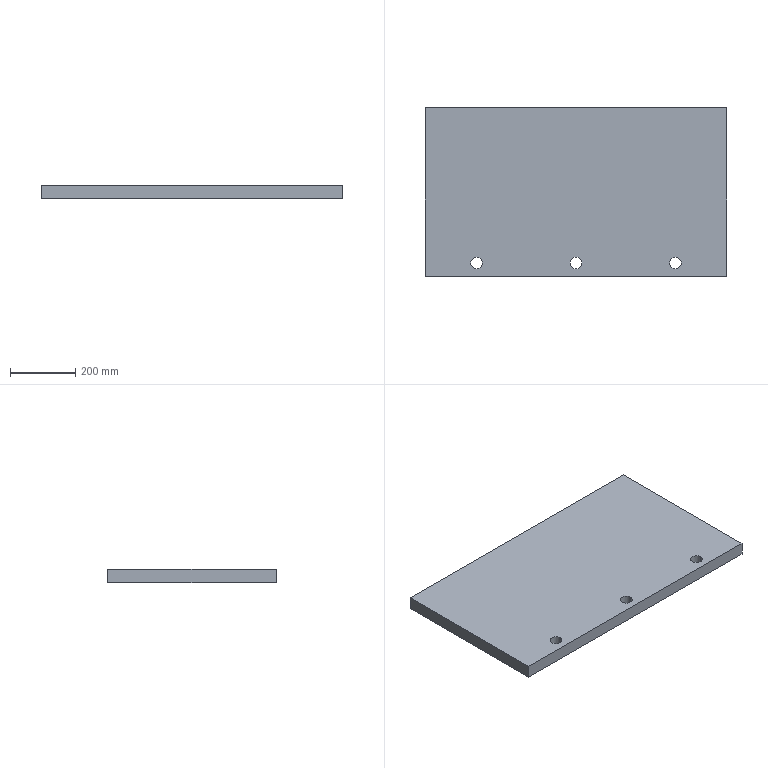Part | SolidWorks | features Extrusion 1 | 1 solid | 12 faces | box 922 x 515 x 40 mm | volume 18871055 mm3 | cylinder 6 | plane 6 | commonest cylinder face diameters 36 x6
STEP:
#1=CARTESIAN_POINT('',(139.,40.,40.));
#2=VERTEX_POINT('',#1);
#3=CARTESIAN_POINT('',(175.,40.,40.));
#4=VERTEX_POINT('',#3);
#5=CARTESIAN_POINT('',(157.,40.,40.));
#6=DIRECTION('',(0.,0.,1.));
#7=DIRECTION('',(1.,0.,0.));
#8=AXIS2_PLACEMENT_3D('',#5,#6,#7);
#9=CIRCLE('',#8,18.);
#10=EDGE_CURVE('',#2,#4,#9,.T.);
#11=ORIENTED_EDGE('',*,*,#10,.T.);
#12=CARTESIAN_POINT('',(175.,40.,0.));
#13=VERTEX_POINT('',#12);
#14=CARTESIAN_POINT('',(175.,40.,40.));
#15=DIRECTION('',(0.,0.,-1.));
#16=VECTOR('',#15,1000.);
#17=LINE('',#14,#16);
#18=EDGE_CURVE('',#4,#13,#17,.T.);
#19=ORIENTED_EDGE('',*,*,#18,.T.);
#20=CARTESIAN_POINT('',(139.,40.,0.));
#21=VERTEX_POINT('',#20);
#22=CARTESIAN_POINT('',(157.,40.,0.));
#23=DIRECTION('',(0.,0.,1.));
#24=DIRECTION('',(1.,0.,0.));
#25=AXIS2_PLACEMENT_3D('',#22,#23,#24);
#26=CIRCLE('',#25,18.);
#27=EDGE_CURVE('',#21,#13,#26,.T.);
#28=ORIENTED_EDGE('',*,*,#27,.F.);
#29=CARTESIAN_POINT('',(139.,40.,40.));
#30=DIRECTION('',(0.,0.,-1.));
#31=VECTOR('',#30,1000.);
#32=LINE('',#29,#31);
#33=EDGE_CURVE('',#2,#21,#32,.T.);
#34=ORIENTED_EDGE('',*,*,#33,.F.);
#35=EDGE_LOOP('',(#11,#19,#28,#34));
#36=FACE_OUTER_BOUND('',#35,.T.);
#37=CARTESIAN_POINT('',(157.,40.,40.));
#38=DIRECTION('',(0.,0.,-1.));
#39=DIRECTION('',(-1.,0.,0.));
#40=AXIS2_PLACEMENT_3D('',#37,#38,#39);
#41=CYLINDRICAL_SURFACE('',#40,18.);
#42=ADVANCED_FACE('',(#36),#41,.F.);
#43=CARTESIAN_POINT('',(747.,40.,40.));
#44=VERTEX_POINT('',#43);
#45=CARTESIAN_POINT('',(783.,40.,40.));
#46=VERTEX_POINT('',#45);
#47=CARTESIAN_POINT('',(765.,40.,40.));
#48=DIRECTION('',(0.,0.,1.));
#49=DIRECTION('',(1.,0.,0.));
#50=AXIS2_PLACEMENT_3D('',#47,#48,#49);
#51=CIRCLE('',#50,18.);
#52=EDGE_CURVE('',#44,#46,#51,.T.);
#53=ORIENTED_EDGE('',*,*,#52,.T.);
#54=CARTESIAN_POINT('',(783.,40.,0.));
#55=VERTEX_POINT('',#54);
#56=CARTESIAN_POINT('',(783.,40.,40.));
#57=DIRECTION('',(0.,0.,-1.));
#58=VECTOR('',#57,1000.);
#59=LINE('',#56,#58);
#60=EDGE_CURVE('',#46,#55,#59,.T.);
#61=ORIENTED_EDGE('',*,*,#60,.T.);
#62=CARTESIAN_POINT('',(747.,40.,0.));
#63=VERTEX_POINT('',#62);
#64=CARTESIAN_POINT('',(765.,40.,0.));
#65=DIRECTION('',(0.,0.,1.));
#66=DIRECTION('',(1.,0.,0.));
#67=AXIS2_PLACEMENT_3D('',#64,#65,#66);
#68=CIRCLE('',#67,18.);
#69=EDGE_CURVE('',#63,#55,#68,.T.);
#70=ORIENTED_EDGE('',*,*,#69,.F.);
#71=CARTESIAN_POINT('',(747.,40.,40.));
#72=DIRECTION('',(0.,0.,-1.));
#73=VECTOR('',#72,1000.);
#74=LINE('',#71,#73);
#75=EDGE_CURVE('',#44,#63,#74,.T.);
#76=ORIENTED_EDGE('',*,*,#75,.F.);
#77=EDGE_LOOP('',(#53,#61,#70,#76));
#78=FACE_OUTER_BOUND('',#77,.T.);
#79=CARTESIAN_POINT('',(765.,40.,40.));
#80=DIRECTION('',(0.,0.,-1.));
#81=DIRECTION('',(-1.,0.,0.));
#82=AXIS2_PLACEMENT_3D('',#79,#80,#81);
#83=CYLINDRICAL_SURFACE('',#82,18.);
#84=ADVANCED_FACE('',(#78),#83,.F.);
#85=CARTESIAN_POINT('',(443.,40.,40.));
#86=VERTEX_POINT('',#85);
#87=CARTESIAN_POINT('',(479.,40.,40.));
#88=VERTEX_POINT('',#87);
#89=CARTESIAN_POINT('',(461.,40.,40.));
#90=DIRECTION('',(0.,0.,1.));
#91=DIRECTION('',(1.,0.,0.));
#92=AXIS2_PLACEMENT_3D('',#89,#90,#91);
#93=CIRCLE('',#92,18.);
#94=EDGE_CURVE('',#86,#88,#93,.T.);
#95=ORIENTED_EDGE('',*,*,#94,.T.);
#96=CARTESIAN_POINT('',(479.,40.,0.));
#97=VERTEX_POINT('',#96);
#98=CARTESIAN_POINT('',(479.,40.,40.));
#99=DIRECTION('',(0.,0.,-1.));
#100=VECTOR('',#99,1000.);
#101=LINE('',#98,#100);
#102=EDGE_CURVE('',#88,#97,#101,.T.);
#103=ORIENTED_EDGE('',*,*,#102,.T.);
#104=CARTESIAN_POINT('',(443.,40.,0.));
#105=VERTEX_POINT('',#104);
#106=CARTESIAN_POINT('',(461.,40.,0.));
#107=DIRECTION('',(0.,0.,1.));
#108=DIRECTION('',(1.,0.,0.));
#109=AXIS2_PLACEMENT_3D('',#106,#107,#108);
#110=CIRCLE('',#109,18.);
#111=EDGE_CURVE('',#105,#97,#110,.T.);
#112=ORIENTED_EDGE('',*,*,#111,.F.);
#113=CARTESIAN_POINT('',(443.,40.,40.));
#114=DIRECTION('',(0.,0.,-1.));
#115=VECTOR('',#114,1000.);
#116=LINE('',#113,#115);
#117=EDGE_CURVE('',#86,#105,#116,.T.);
#118=ORIENTED_EDGE('',*,*,#117,.F.);
#119=EDGE_LOOP('',(#95,#103,#112,#118));
#120=FACE_OUTER_BOUND('',#119,.T.);
#121=CARTESIAN_POINT('',(461.,40.,40.));
#122=DIRECTION('',(0.,0.,-1.));
#123=DIRECTION('',(-1.,0.,0.));
#124=AXIS2_PLACEMENT_3D('',#121,#122,#123);
#125=CYLINDRICAL_SURFACE('',#124,18.);
#126=ADVANCED_FACE('',(#120),#125,.F.);
#127=CARTESIAN_POINT('',(0.,515.,40.));
#128=VERTEX_POINT('',#127);
#129=CARTESIAN_POINT('',(0.,0.,40.));
#130=VERTEX_POINT('',#129);
#131=CARTESIAN_POINT('',(0.,0.,40.));
#132=DIRECTION('',(0.,-1.,0.));
#133=VECTOR('',#132,1000.);
#134=LINE('',#131,#133);
#135=EDGE_CURVE('',#128,#130,#134,.T.);
#136=ORIENTED_EDGE('',*,*,#135,.T.);
#137=CARTESIAN_POINT('',(922.,0.,40.));
#138=VERTEX_POINT('',#137);
#139=CARTESIAN_POINT('',(0.,0.,40.));
#140=DIRECTION('',(1.,0.,0.));
#141=VECTOR('',#140,1000.);
#142=LINE('',#139,#141);
#143=EDGE_CURVE('',#130,#138,#142,.T.);
#144=ORIENTED_EDGE('',*,*,#143,.T.);
#145=CARTESIAN_POINT('',(922.,515.,40.));
#146=VERTEX_POINT('',#145);
#147=CARTESIAN_POINT('',(922.,0.,40.));
#148=DIRECTION('',(0.,1.,0.));
#149=VECTOR('',#148,1000.);
#150=LINE('',#147,#149);
#151=EDGE_CURVE('',#138,#146,#150,.T.);
#152=ORIENTED_EDGE('',*,*,#151,.T.);
#153=CARTESIAN_POINT('',(0.,515.,40.));
#154=DIRECTION('',(-1.,0.,0.));
#155=VECTOR('',#154,1000.);
#156=LINE('',#153,#155);
#157=EDGE_CURVE('',#146,#128,#156,.T.);
#158=ORIENTED_EDGE('',*,*,#157,.T.);
#159=EDGE_LOOP('',(#136,#144,#152,#158));
#160=FACE_OUTER_BOUND('',#159,.T.);
#161=ORIENTED_EDGE('',*,*,#94,.F.);
#162=CARTESIAN_POINT('',(461.,40.,40.));
#163=DIRECTION('',(0.,0.,1.));
#164=DIRECTION('',(1.,0.,0.));
#165=AXIS2_PLACEMENT_3D('',#162,#163,#164);
#166=CIRCLE('',#165,18.);
#167=EDGE_CURVE('',#88,#86,#166,.T.);
#168=ORIENTED_EDGE('',*,*,#167,.F.);
#169=EDGE_LOOP('',(#161,#168));
#170=FACE_BOUND('',#169,.T.);
#171=ORIENTED_EDGE('',*,*,#52,.F.);
#172=CARTESIAN_POINT('',(765.,40.,40.));
#173=DIRECTION('',(0.,0.,1.));
#174=DIRECTION('',(1.,0.,0.));
#175=AXIS2_PLACEMENT_3D('',#172,#173,#174);
#176=CIRCLE('',#175,18.);
#177=EDGE_CURVE('',#46,#44,#176,.T.);
#178=ORIENTED_EDGE('',*,*,#177,.F.);
#179=EDGE_LOOP('',(#171,#178));
#180=FACE_BOUND('',#179,.T.);
#181=ORIENTED_EDGE('',*,*,#10,.F.);
#182=CARTESIAN_POINT('',(157.,40.,40.));
#183=DIRECTION('',(0.,0.,1.));
#184=DIRECTION('',(1.,0.,0.));
#185=AXIS2_PLACEMENT_3D('',#182,#183,#184);
#186=CIRCLE('',#185,18.);
#187=EDGE_CURVE('',#4,#2,#186,.T.);
#188=ORIENTED_EDGE('',*,*,#187,.F.);
#189=EDGE_LOOP('',(#181,#188));
#190=FACE_BOUND('',#189,.T.);
#191=CARTESIAN_POINT('',(0.,0.,40.));
#192=DIRECTION('',(0.,0.,-1.));
#193=DIRECTION('',(-1.,0.,0.));
#194=AXIS2_PLACEMENT_3D('',#191,#192,#193);
#195=PLANE('',#194);
#196=ADVANCED_FACE('',(#160,#170,#180,#190),#195,.F.);
#197=ORIENTED_EDGE('',*,*,#69,.T.);
#198=CARTESIAN_POINT('',(765.,40.,0.));
#199=DIRECTION('',(0.,0.,1.));
#200=DIRECTION('',(1.,0.,0.));
#201=AXIS2_PLACEMENT_3D('',#198,#199,#200);
#202=CIRCLE('',#201,18.);
#203=EDGE_CURVE('',#55,#63,#202,.T.);
#204=ORIENTED_EDGE('',*,*,#203,.T.);
#205=EDGE_LOOP('',(#197,#204));
#206=FACE_BOUND('',#205,.T.);
#207=CARTESIAN_POINT('',(0.,515.,0.));
#208=VERTEX_POINT('',#207);
#209=CARTESIAN_POINT('',(0.,0.,0.));
#210=VERTEX_POINT('',#209);
#211=CARTESIAN_POINT('',(0.,0.,0.));
#212=DIRECTION('',(0.,-1.,0.));
#213=VECTOR('',#212,1000.);
#214=LINE('',#211,#213);
#215=EDGE_CURVE('',#208,#210,#214,.T.);
#216=ORIENTED_EDGE('',*,*,#215,.F.);
#217=CARTESIAN_POINT('',(922.,515.,0.));
#218=VERTEX_POINT('',#217);
#219=CARTESIAN_POINT('',(0.,515.,0.));
#220=DIRECTION('',(-1.,0.,0.));
#221=VECTOR('',#220,1000.);
#222=LINE('',#219,#221);
#223=EDGE_CURVE('',#218,#208,#222,.T.);
#224=ORIENTED_EDGE('',*,*,#223,.F.);
#225=CARTESIAN_POINT('',(922.,0.,0.));
#226=VERTEX_POINT('',#225);
#227=CARTESIAN_POINT('',(922.,0.,0.));
#228=DIRECTION('',(0.,1.,0.));
#229=VECTOR('',#228,1000.);
#230=LINE('',#227,#229);
#231=EDGE_CURVE('',#226,#218,#230,.T.);
#232=ORIENTED_EDGE('',*,*,#231,.F.);
#233=CARTESIAN_POINT('',(0.,0.,0.));
#234=DIRECTION('',(1.,0.,0.));
#235=VECTOR('',#234,1000.);
#236=LINE('',#233,#235);
#237=EDGE_CURVE('',#210,#226,#236,.T.);
#238=ORIENTED_EDGE('',*,*,#237,.F.);
#239=EDGE_LOOP('',(#216,#224,#232,#238));
#240=FACE_OUTER_BOUND('',#239,.T.);
#241=ORIENTED_EDGE('',*,*,#111,.T.);
#242=CARTESIAN_POINT('',(461.,40.,0.));
#243=DIRECTION('',(0.,0.,1.));
#244=DIRECTION('',(1.,0.,0.));
#245=AXIS2_PLACEMENT_3D('',#242,#243,#244);
#246=CIRCLE('',#245,18.);
#247=EDGE_CURVE('',#97,#105,#246,.T.);
#248=ORIENTED_EDGE('',*,*,#247,.T.);
#249=EDGE_LOOP('',(#241,#248));
#250=FACE_BOUND('',#249,.T.);
#251=ORIENTED_EDGE('',*,*,#27,.T.);
#252=CARTESIAN_POINT('',(157.,40.,0.));
#253=DIRECTION('',(0.,0.,1.));
#254=DIRECTION('',(1.,0.,0.));
#255=AXIS2_PLACEMENT_3D('',#252,#253,#254);
#256=CIRCLE('',#255,18.);
#257=EDGE_CURVE('',#13,#21,#256,.T.);
#258=ORIENTED_EDGE('',*,*,#257,.T.);
#259=EDGE_LOOP('',(#251,#258));
#260=FACE_BOUND('',#259,.T.);
#261=CARTESIAN_POINT('',(0.,0.,0.));
#262=DIRECTION('',(0.,0.,-1.));
#263=DIRECTION('',(-1.,0.,0.));
#264=AXIS2_PLACEMENT_3D('',#261,#262,#263);
#265=PLANE('',#264);
#266=ADVANCED_FACE('',(#206,#240,#250,#260),#265,.T.);
#267=ORIENTED_EDGE('',*,*,#215,.T.);
#268=CARTESIAN_POINT('',(0.,0.,40.));
#269=DIRECTION('',(0.,0.,-1.));
#270=VECTOR('',#269,1000.);
#271=LINE('',#268,#270);
#272=EDGE_CURVE('',#130,#210,#271,.T.);
#273=ORIENTED_EDGE('',*,*,#272,.F.);
#274=ORIENTED_EDGE('',*,*,#135,.F.);
#275=CARTESIAN_POINT('',(0.,515.,40.));
#276=DIRECTION('',(0.,0.,-1.));
#277=VECTOR('',#276,1000.);
#278=LINE('',#275,#277);
#279=EDGE_CURVE('',#128,#208,#278,.T.);
#280=ORIENTED_EDGE('',*,*,#279,.T.);
#281=EDGE_LOOP('',(#267,#273,#274,#280));
#282=FACE_OUTER_BOUND('',#281,.T.);
#283=CARTESIAN_POINT('',(0.,0.,40.));
#284=DIRECTION('',(1.,0.,0.));
#285=DIRECTION('',(0.,0.,-1.));
#286=AXIS2_PLACEMENT_3D('',#283,#284,#285);
#287=PLANE('',#286);
#288=ADVANCED_FACE('',(#282),#287,.F.);
#289=ORIENTED_EDGE('',*,*,#237,.T.);
#290=CARTESIAN_POINT('',(922.,0.,40.));
#291=DIRECTION('',(0.,0.,-1.));
#292=VECTOR('',#291,1000.);
#293=LINE('',#290,#292);
#294=EDGE_CURVE('',#138,#226,#293,.T.);
#295=ORIENTED_EDGE('',*,*,#294,.F.);
#296=ORIENTED_EDGE('',*,*,#143,.F.);
#297=ORIENTED_EDGE('',*,*,#272,.T.);
#298=EDGE_LOOP('',(#289,#295,#296,#297));
#299=FACE_OUTER_BOUND('',#298,.T.);
#300=CARTESIAN_POINT('',(0.,0.,40.));
#301=DIRECTION('',(0.,1.,0.));
#302=DIRECTION('',(0.,0.,1.));
#303=AXIS2_PLACEMENT_3D('',#300,#301,#302);
#304=PLANE('',#303);
#305=ADVANCED_FACE('',(#299),#304,.F.);
#306=ORIENTED_EDGE('',*,*,#231,.T.);
#307=CARTESIAN_POINT('',(922.,515.,40.));
#308=DIRECTION('',(0.,0.,-1.));
#309=VECTOR('',#308,1000.);
#310=LINE('',#307,#309);
#311=EDGE_CURVE('',#146,#218,#310,.T.);
#312=ORIENTED_EDGE('',*,*,#311,.F.);
#313=ORIENTED_EDGE('',*,*,#151,.F.);
#314=ORIENTED_EDGE('',*,*,#294,.T.);
#315=EDGE_LOOP('',(#306,#312,#313,#314));
#316=FACE_OUTER_BOUND('',#315,.T.);
#317=CARTESIAN_POINT('',(922.,0.,40.));
#318=DIRECTION('',(-1.,0.,0.));
#319=DIRECTION('',(0.,0.,1.));
#320=AXIS2_PLACEMENT_3D('',#317,#318,#319);
#321=PLANE('',#320);
#322=ADVANCED_FACE('',(#316),#321,.F.);
#323=ORIENTED_EDGE('',*,*,#223,.T.);
#324=ORIENTED_EDGE('',*,*,#279,.F.);
#325=ORIENTED_EDGE('',*,*,#157,.F.);
#326=ORIENTED_EDGE('',*,*,#311,.T.);
#327=EDGE_LOOP('',(#323,#324,#325,#326));
#328=FACE_OUTER_BOUND('',#327,.T.);
#329=CARTESIAN_POINT('',(0.,515.,40.));
#330=DIRECTION('',(0.,-1.,0.));
#331=DIRECTION('',(0.,0.,-1.));
#332=AXIS2_PLACEMENT_3D('',#329,#330,#331);
#333=PLANE('',#332);
#334=ADVANCED_FACE('',(#328),#333,.F.);
#335=ORIENTED_EDGE('',*,*,#102,.F.);
#336=ORIENTED_EDGE('',*,*,#167,.T.);
#337=ORIENTED_EDGE('',*,*,#117,.T.);
#338=ORIENTED_EDGE('',*,*,#247,.F.);
#339=EDGE_LOOP('',(#335,#336,#337,#338));
#340=FACE_OUTER_BOUND('',#339,.T.);
#341=CARTESIAN_POINT('',(461.,40.,40.));
#342=DIRECTION('',(0.,0.,-1.));
#343=DIRECTION('',(-1.,0.,0.));
#344=AXIS2_PLACEMENT_3D('',#341,#342,#343);
#345=CYLINDRICAL_SURFACE('',#344,18.);
#346=ADVANCED_FACE('',(#340),#345,.F.);
#347=ORIENTED_EDGE('',*,*,#60,.F.);
#348=ORIENTED_EDGE('',*,*,#177,.T.);
#349=ORIENTED_EDGE('',*,*,#75,.T.);
#350=ORIENTED_EDGE('',*,*,#203,.F.);
#351=EDGE_LOOP('',(#347,#348,#349,#350));
#352=FACE_OUTER_BOUND('',#351,.T.);
#353=CARTESIAN_POINT('',(765.,40.,40.));
#354=DIRECTION('',(0.,0.,-1.));
#355=DIRECTION('',(-1.,0.,0.));
#356=AXIS2_PLACEMENT_3D('',#353,#354,#355);
#357=CYLINDRICAL_SURFACE('',#356,18.);
#358=ADVANCED_FACE('',(#352),#357,.F.);
#359=ORIENTED_EDGE('',*,*,#18,.F.);
#360=ORIENTED_EDGE('',*,*,#187,.T.);
#361=ORIENTED_EDGE('',*,*,#33,.T.);
#362=ORIENTED_EDGE('',*,*,#257,.F.);
#363=EDGE_LOOP('',(#359,#360,#361,#362));
#364=FACE_OUTER_BOUND('',#363,.T.);
#365=CARTESIAN_POINT('',(157.,40.,40.));
#366=DIRECTION('',(0.,0.,-1.));
#367=DIRECTION('',(-1.,0.,0.));
#368=AXIS2_PLACEMENT_3D('',#365,#366,#367);
#369=CYLINDRICAL_SURFACE('',#368,18.);
#370=ADVANCED_FACE('',(#364),#369,.F.);
#371=CLOSED_SHELL('',(#42,#84,#126,#196,#266,#288,#305,#322,#334,#346,#358,#370));
#372=MANIFOLD_SOLID_BREP('',#371);
#373=CARTESIAN_POINT('',(0.,0.,0.));
#374=DIRECTION('',(0.,0.,1.));
#375=DIRECTION('',(1.,0.,0.));
#376=AXIS2_PLACEMENT_3D('',#373,#374,#375);
#377=(LENGTH_UNIT()NAMED_UNIT(*)SI_UNIT(.MILLI.,.METRE.));
#378=UNCERTAINTY_MEASURE_WITH_UNIT(LENGTH_MEASURE(0.00001),#377,'','');
#379=(NAMED_UNIT(*)PLANE_ANGLE_UNIT()SI_UNIT($,.RADIAN.));
#380=(NAMED_UNIT(*)SI_UNIT($,.STERADIAN.)SOLID_ANGLE_UNIT());
#381=(GEOMETRIC_REPRESENTATION_CONTEXT(3)GLOBAL_UNCERTAINTY_ASSIGNED_CONTEXT((#378))GLOBAL_UNIT_ASSIGNED_CONTEXT((#377,#379,#380))REPRESENTATION_CONTEXT('',''));
#382=ADVANCED_BREP_SHAPE_REPRESENTATION('',(#372,#376),#381);